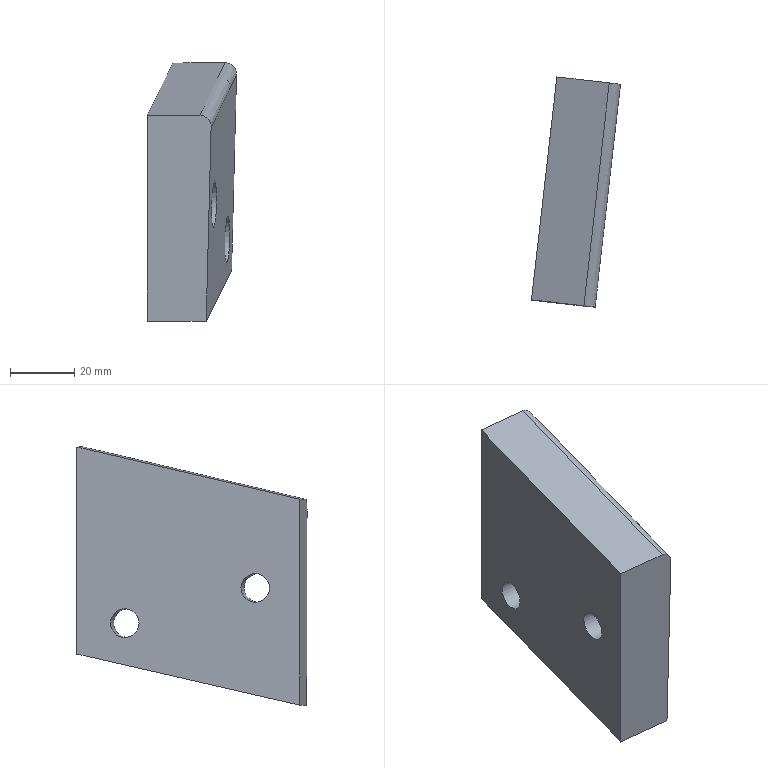Part | NX | features 23 2 | 1 solid | 13 faces | box 27.795 x 71.813 x 80.626 mm | volume 82272 mm3 | plane 7 | cylinder 4 | spline 2 | commonest cylinder face diameters 9 x2 14.5 x2
STEP:
#1=CARTESIAN_POINT('',(2638.723,-314.145,-117.631));
#2=VERTEX_POINT('',#1);
#3=CARTESIAN_POINT('',(2646.647,-244.595,-101.684));
#4=VERTEX_POINT('',#3);
#5=CARTESIAN_POINT('',(2657.951,-145.383,-78.935));
#6=DIRECTION('',(0.1104,0.9687,0.2221));
#7=VECTOR('',#6,1000.);
#8=LINE('',#5,#7);
#9=EDGE_CURVE('',#2,#4,#8,.T.);
#10=ORIENTED_EDGE('',*,*,#9,.T.);
#11=CARTESIAN_POINT('',(2648.194,-244.771,-40.694));
#12=VERTEX_POINT('',#11);
#13=CARTESIAN_POINT('',(2646.722,-244.604,-98.712));
#14=DIRECTION('',(0.02536,-0.002889,0.9997));
#15=VECTOR('',#14,1000.);
#16=LINE('',#13,#15);
#17=EDGE_CURVE('',#4,#12,#16,.T.);
#18=ORIENTED_EDGE('',*,*,#17,.T.);
#19=CARTESIAN_POINT('',(2640.259,-314.32,-57.071));
#20=VERTEX_POINT('',#19);
#21=CARTESIAN_POINT('',(2648.194,-244.771,-40.694));
#22=CARTESIAN_POINT('',(2648.121,-245.409,-40.844));
#23=CARTESIAN_POINT('',(2647.971,-246.727,-41.154));
#24=CARTESIAN_POINT('',(2647.771,-248.484,-41.566));
#25=CARTESIAN_POINT('',(2647.603,-249.954,-41.911));
#26=CARTESIAN_POINT('',(2647.473,-251.092,-42.178));
#27=CARTESIAN_POINT('',(2647.363,-252.06,-42.405));
#28=CARTESIAN_POINT('',(2647.282,-252.767,-42.571));
#29=CARTESIAN_POINT('',(2647.238,-253.152,-42.661));
#30=CARTESIAN_POINT('',(2647.197,-253.509,-42.744));
#31=CARTESIAN_POINT('',(2647.186,-253.611,-42.768));
#32=CARTESIAN_POINT('',(2647.159,-253.849,-42.824));
#33=CARTESIAN_POINT('',(2647.113,-254.247,-42.917));
#34=CARTESIAN_POINT('',(2647.037,-254.913,-43.073));
#35=CARTESIAN_POINT('',(2646.934,-255.821,-43.285));
#36=CARTESIAN_POINT('',(2646.778,-257.19,-43.605));
#37=CARTESIAN_POINT('',(2646.593,-258.809,-43.984));
#38=CARTESIAN_POINT('',(2646.386,-260.625,-44.409));
#39=CARTESIAN_POINT('',(2646.205,-262.211,-44.779));
#40=CARTESIAN_POINT('',(2646.057,-263.51,-45.083));
#41=CARTESIAN_POINT('',(2645.862,-265.219,-45.483));
#42=CARTESIAN_POINT('',(2645.642,-267.144,-45.933));
#43=CARTESIAN_POINT('',(2645.448,-268.843,-46.331));
#44=CARTESIAN_POINT('',(2645.33,-269.883,-46.574));
#45=CARTESIAN_POINT('',(2645.263,-270.472,-46.712));
#46=CARTESIAN_POINT('',(2645.224,-270.807,-46.791));
#47=CARTESIAN_POINT('',(2645.15,-271.46,-46.944));
#48=CARTESIAN_POINT('',(2645.064,-272.21,-47.119));
#49=CARTESIAN_POINT('',(2644.911,-273.556,-47.435));
#50=CARTESIAN_POINT('',(2644.701,-275.393,-47.867));
#51=CARTESIAN_POINT('',(2644.497,-277.181,-48.287));
#52=CARTESIAN_POINT('',(2644.343,-278.535,-48.606));
#53=CARTESIAN_POINT('',(2644.22,-279.609,-48.859));
#54=CARTESIAN_POINT('',(2644.135,-280.355,-49.034));
#55=CARTESIAN_POINT('',(2644.002,-281.523,-49.31));
#56=CARTESIAN_POINT('',(2643.761,-283.631,-49.808));
#57=CARTESIAN_POINT('',(2643.374,-287.024,-50.609));
#58=CARTESIAN_POINT('',(2642.933,-290.886,-51.523));
#59=CARTESIAN_POINT('',(2642.599,-293.818,-52.217));
#60=CARTESIAN_POINT('',(2642.396,-295.596,-52.638));
#61=CARTESIAN_POINT('',(2642.25,-296.876,-52.941));
#62=CARTESIAN_POINT('',(2642.061,-298.527,-53.333));
#63=CARTESIAN_POINT('',(2641.837,-300.493,-53.798));
#64=CARTESIAN_POINT('',(2641.569,-302.845,-54.355));
#65=CARTESIAN_POINT('',(2641.278,-305.392,-54.958));
#66=CARTESIAN_POINT('',(2640.928,-308.459,-55.684));
#67=CARTESIAN_POINT('',(2640.563,-311.658,-56.442));
#68=CARTESIAN_POINT('',(2640.347,-313.545,-56.888));
#69=CARTESIAN_POINT('',(2640.259,-314.32,-57.071));
#70=B_SPLINE_CURVE_WITH_KNOTS('',3,(#21,#22,#23,#24,#25,#26,#27,#28,#29,#30,#31,#32,#33,#34,#35,#36,#37,#38,#39,#40,#41,#42,#43,#44,#45,#46,#47,#48,#49,#50,#51,#52,#53,#54,#55,#56,#57,#58,#59,#60,#61,#62,#63,#64,#65,#66,#67,#68,#69),.UNSPECIFIED.,.F.,.F.,(4,1,1,1,1,1,1,1,1,1,1,1,1,1,1,1,1,1,1,1,1,1,1,1,1,1,1,1,1,1,1,1,1,1,1,1,1,1,1,1,1,1,1,1,1,1,4),(0.,0.03125,0.0625,0.07812,0.09375,0.1094,0.1172,0.1211,0.125,0.1289,0.1328,0.1406,0.1562,0.1719,0.1875,0.2188,0.2344,0.25,0.2656,0.2812,0.3125,0.3438,0.3594,0.3672,0.375,0.3828,0.3906,0.4062,0.4375,0.4688,0.4844,0.5,0.5156,0.5312,0.5625,0.625,0.6875,0.7188,0.7344,0.75,0.7656,0.7812,0.8125,0.8438,0.875,0.9375,1.),.UNSPECIFIED.);
#71=EDGE_CURVE('',#20,#12,#70,.F.);
#72=ORIENTED_EDGE('',*,*,#71,.F.);
#73=CARTESIAN_POINT('',(2639.202,-314.2,-98.722));
#74=DIRECTION('',(0.02536,-0.002889,0.9997));
#75=VECTOR('',#74,1000.);
#76=LINE('',#73,#75);
#77=EDGE_CURVE('',#2,#20,#76,.T.);
#78=ORIENTED_EDGE('',*,*,#77,.F.);
#79=EDGE_LOOP('',(#10,#18,#72,#78));
#80=FACE_BOUND('',#79,.T.);
#81=CARTESIAN_POINT('',(2641.148,-298.71,-88.121));
#82=VERTEX_POINT('',#81);
#83=CARTESIAN_POINT('',(2641.155,-300.332,-81.052));
#84=DIRECTION('',(0.9939,-0.1074,-0.02552));
#85=DIRECTION('',(-0.0008715,0.2236,-0.9747));
#86=AXIS2_PLACEMENT_3D('',#83,#84,#85);
#87=ELLIPSE('',#86,7.252,7.25);
#88=EDGE_CURVE('',#82,#82,#87,.T.);
#89=ORIENTED_EDGE('',*,*,#88,.F.);
#90=EDGE_LOOP('',(#89));
#91=FACE_BOUND('',#90,.T.);
#92=CARTESIAN_POINT('',(2645.274,-257.915,-99.121));
#93=VERTEX_POINT('',#92);
#94=CARTESIAN_POINT('',(2645.28,-259.536,-92.052));
#95=DIRECTION('',(-0.9939,0.1074,0.02552));
#96=DIRECTION('',(-0.0008715,0.2236,-0.9747));
#97=AXIS2_PLACEMENT_3D('',#94,#95,#96);
#98=ELLIPSE('',#97,7.252,7.25);
#99=EDGE_CURVE('',#93,#93,#98,.T.);
#100=ORIENTED_EDGE('',*,*,#99,.T.);
#101=EDGE_LOOP('',(#100));
#102=FACE_BOUND('',#101,.T.);
#103=CARTESIAN_POINT('',(2489.055,-1559.415,-706.392));
#104=DIRECTION('',(0.9939,-0.1074,-0.02552));
#105=DIRECTION('',(-0.02537,0.002816,-0.9997));
#106=AXIS2_PLACEMENT_3D('',#103,#104,#105);
#107=PLANE('',#106);
#108=ADVANCED_FACE('',(#80,#91,#102),#107,.T.);
#109=CARTESIAN_POINT('',(2620.4,-312.058,-117.631));
#110=VERTEX_POINT('',#109);
#111=CARTESIAN_POINT('',(2630.336,-313.19,-117.631));
#112=DIRECTION('',(-0.9936,0.1132,-0.000000001));
#113=VECTOR('',#112,1000.);
#114=LINE('',#111,#113);
#115=EDGE_CURVE('',#2,#110,#114,.T.);
#116=ORIENTED_EDGE('',*,*,#115,.F.);
#117=ORIENTED_EDGE('',*,*,#77,.T.);
#118=CARTESIAN_POINT('',(2636.764,-313.922,-53.382));
#119=VERTEX_POINT('',#118);
#120=CARTESIAN_POINT('',(2636.764,-313.922,-53.382));
#121=CARTESIAN_POINT('',(2637.715,-314.03,-53.377));
#122=CARTESIAN_POINT('',(2639.568,-314.242,-54.211));
#123=CARTESIAN_POINT('',(2640.283,-314.323,-56.116));
#124=CARTESIAN_POINT('',(2640.259,-314.32,-57.071));
#125=B_SPLINE_CURVE_WITH_KNOTS('',3,(#120,#121,#122,#123,#124),.UNSPECIFIED.,.F.,.F.,(4,1,4),(0.,0.002827,0.005655),.UNSPECIFIED.);
#126=EDGE_CURVE('',#119,#20,#125,.T.);
#127=ORIENTED_EDGE('',*,*,#126,.F.);
#128=CARTESIAN_POINT('',(2620.4,-312.058,-53.345));
#129=VERTEX_POINT('',#128);
#130=CARTESIAN_POINT('',(2636.764,-313.922,-53.382));
#131=CARTESIAN_POINT('',(2631.31,-313.301,-53.411));
#132=CARTESIAN_POINT('',(2625.855,-312.679,-53.392));
#133=CARTESIAN_POINT('',(2620.4,-312.058,-53.345));
#134=B_SPLINE_CURVE_WITH_KNOTS('',3,(#130,#131,#132,#133),.UNSPECIFIED.,.F.,.F.,(4,4),(0.,0.01647),.UNSPECIFIED.);
#135=EDGE_CURVE('',#119,#129,#134,.T.);
#136=ORIENTED_EDGE('',*,*,#135,.T.);
#137=CARTESIAN_POINT('',(2620.4,-312.058,-77.534));
#138=DIRECTION('',(-0.000000001,0.,1.));
#139=VECTOR('',#138,1000.);
#140=LINE('',#137,#139);
#141=EDGE_CURVE('',#110,#129,#140,.T.);
#142=ORIENTED_EDGE('',*,*,#141,.F.);
#143=EDGE_LOOP('',(#116,#117,#127,#136,#142));
#144=FACE_BOUND('',#143,.T.);
#145=CARTESIAN_POINT('',(2630.336,-313.19,-98.495));
#146=DIRECTION('',(-0.1132,-0.9936,0.));
#147=DIRECTION('',(-0.9936,0.1132,0.));
#148=AXIS2_PLACEMENT_3D('',#145,#146,#147);
#149=PLANE('',#148);
#150=ADVANCED_FACE('',(#144),#149,.T.);
#151=CARTESIAN_POINT('',(2627.135,-252.94,-92.052));
#152=VERTEX_POINT('',#151);
#153=CARTESIAN_POINT('',(2626.626,-257.411,-92.052));
#154=DIRECTION('',(0.9936,-0.1132,0.000000001));
#155=DIRECTION('',(0.1132,0.9936,0.));
#156=AXIS2_PLACEMENT_3D('',#153,#154,#155);
#157=CIRCLE('',#156,4.5);
#158=EDGE_CURVE('',#152,#152,#157,.T.);
#159=ORIENTED_EDGE('',*,*,#158,.T.);
#160=EDGE_LOOP('',(#159));
#161=FACE_BOUND('',#160,.T.);
#162=CARTESIAN_POINT('',(2622.494,-293.677,-81.052));
#163=VERTEX_POINT('',#162);
#164=CARTESIAN_POINT('',(2621.985,-298.148,-81.052));
#165=DIRECTION('',(0.9936,-0.1132,0.000000001));
#166=DIRECTION('',(0.1132,0.9936,0.));
#167=AXIS2_PLACEMENT_3D('',#164,#165,#166);
#168=CIRCLE('',#167,4.5);
#169=EDGE_CURVE('',#163,#163,#168,.T.);
#170=ORIENTED_EDGE('',*,*,#169,.T.);
#171=EDGE_LOOP('',(#170));
#172=FACE_BOUND('',#171,.T.);
#173=CARTESIAN_POINT('',(2628.324,-242.508,-101.684));
#174=VERTEX_POINT('',#173);
#175=CARTESIAN_POINT('',(2628.324,-242.508,-37.059));
#176=VERTEX_POINT('',#175);
#177=CARTESIAN_POINT('',(2628.324,-242.508,-77.534));
#178=DIRECTION('',(-0.000000001,0.,1.));
#179=VECTOR('',#178,1000.);
#180=LINE('',#177,#179);
#181=EDGE_CURVE('',#174,#176,#180,.T.);
#182=ORIENTED_EDGE('',*,*,#181,.F.);
#183=CARTESIAN_POINT('',(2624.635,-274.889,-109.109));
#184=DIRECTION('',(0.1104,0.9687,0.2221));
#185=VECTOR('',#184,1000.);
#186=LINE('',#183,#185);
#187=EDGE_CURVE('',#110,#174,#186,.T.);
#188=ORIENTED_EDGE('',*,*,#187,.F.);
#189=ORIENTED_EDGE('',*,*,#141,.T.);
#190=CARTESIAN_POINT('',(2628.324,-242.508,-37.059));
#191=CARTESIAN_POINT('',(2627.663,-248.306,-38.406));
#192=CARTESIAN_POINT('',(2626.341,-259.917,-41.034));
#193=CARTESIAN_POINT('',(2623.701,-283.087,-46.522));
#194=CARTESIAN_POINT('',(2621.72,-300.469,-50.618));
#195=CARTESIAN_POINT('',(2620.4,-312.058,-53.345));
#196=B_SPLINE_CURVE_WITH_KNOTS('',3,(#190,#191,#192,#193,#194,#195),.UNSPECIFIED.,.F.,.F.,(4,1,1,4),(0.000000002,0.01797,0.03593,0.07187),.UNSPECIFIED.);
#197=EDGE_CURVE('',#176,#129,#196,.T.);
#198=ORIENTED_EDGE('',*,*,#197,.F.);
#199=EDGE_LOOP('',(#182,#188,#189,#198));
#200=FACE_BOUND('',#199,.T.);
#201=CARTESIAN_POINT('',(2623.82,-282.036,-77.534));
#202=DIRECTION('',(0.9936,-0.1132,0.000000001));
#203=DIRECTION('',(-0.1132,-0.9936,0.));
#204=AXIS2_PLACEMENT_3D('',#201,#202,#203);
#205=PLANE('',#204);
#206=ADVANCED_FACE('',(#161,#172,#200),#205,.F.);
#207=CARTESIAN_POINT('',(2644.678,-244.371,-37.006));
#208=VERTEX_POINT('',#207);
#209=CARTESIAN_POINT('',(2636.764,-313.922,-53.382));
#210=CARTESIAN_POINT('',(2638.082,-302.336,-50.646));
#211=CARTESIAN_POINT('',(2640.727,-279.163,-45.124));
#212=CARTESIAN_POINT('',(2643.34,-255.967,-39.737));
#213=CARTESIAN_POINT('',(2644.678,-244.371,-37.006));
#214=B_SPLINE_CURVE_WITH_KNOTS('',3,(#209,#210,#211,#212,#213),.UNSPECIFIED.,.F.,.F.,(4,1,4),(0.,0.5,1.),.UNSPECIFIED.);
#215=EDGE_CURVE('',#208,#119,#214,.F.);
#216=ORIENTED_EDGE('',*,*,#215,.F.);
#217=CARTESIAN_POINT('',(2628.324,-242.508,-37.059));
#218=CARTESIAN_POINT('',(2633.775,-243.129,-37.117));
#219=CARTESIAN_POINT('',(2639.227,-243.75,-37.071));
#220=CARTESIAN_POINT('',(2644.678,-244.371,-37.006));
#221=B_SPLINE_CURVE_WITH_KNOTS('',3,(#217,#218,#219,#220),.UNSPECIFIED.,.F.,.F.,(4,4),(0.,0.01646),.UNSPECIFIED.);
#222=EDGE_CURVE('',#176,#208,#221,.T.);
#223=ORIENTED_EDGE('',*,*,#222,.F.);
#224=ORIENTED_EDGE('',*,*,#197,.T.);
#225=ORIENTED_EDGE('',*,*,#135,.F.);
#226=EDGE_LOOP('',(#216,#223,#224,#225));
#227=FACE_BOUND('',#226,.T.);
#228=CARTESIAN_POINT('',(2644.824,-243.965,-36.906));
#229=CARTESIAN_POINT('',(2644.153,-249.833,-38.289));
#230=CARTESIAN_POINT('',(2643.486,-255.702,-39.662));
#231=CARTESIAN_POINT('',(2642.16,-267.439,-42.407));
#232=CARTESIAN_POINT('',(2641.507,-273.309,-43.776));
#233=CARTESIAN_POINT('',(2640.197,-285.036,-46.537));
#234=CARTESIAN_POINT('',(2639.534,-290.893,-47.936));
#235=CARTESIAN_POINT('',(2638.207,-302.63,-50.718));
#236=CARTESIAN_POINT('',(2637.547,-308.495,-52.095));
#237=CARTESIAN_POINT('',(2636.886,-314.358,-53.479));
#238=CARTESIAN_POINT('',(2642.06,-243.64,-36.937));
#239=CARTESIAN_POINT('',(2641.388,-249.513,-38.32));
#240=CARTESIAN_POINT('',(2640.719,-255.386,-39.686));
#241=CARTESIAN_POINT('',(2639.393,-267.125,-42.423));
#242=CARTESIAN_POINT('',(2638.747,-272.992,-43.795));
#243=CARTESIAN_POINT('',(2637.441,-284.719,-46.561));
#244=CARTESIAN_POINT('',(2636.768,-290.578,-47.959));
#245=CARTESIAN_POINT('',(2635.44,-302.314,-50.736));
#246=CARTESIAN_POINT('',(2634.787,-308.182,-52.111));
#247=CARTESIAN_POINT('',(2634.124,-314.045,-53.494));
#248=CARTESIAN_POINT('',(2639.303,-243.311,-36.973));
#249=CARTESIAN_POINT('',(2638.631,-249.192,-38.36));
#250=CARTESIAN_POINT('',(2637.957,-255.074,-39.718));
#251=CARTESIAN_POINT('',(2636.624,-266.814,-42.437));
#252=CARTESIAN_POINT('',(2635.971,-272.67,-43.814));
#253=CARTESIAN_POINT('',(2634.658,-284.398,-46.591));
#254=CARTESIAN_POINT('',(2633.99,-290.265,-47.98));
#255=CARTESIAN_POINT('',(2632.667,-301.996,-50.751));
#256=CARTESIAN_POINT('',(2632.013,-307.864,-52.135));
#257=CARTESIAN_POINT('',(2631.351,-313.73,-53.515));
#258=CARTESIAN_POINT('',(2633.743,-242.67,-36.996));
#259=CARTESIAN_POINT('',(2633.063,-248.562,-38.386));
#260=CARTESIAN_POINT('',(2632.386,-254.454,-39.727));
#261=CARTESIAN_POINT('',(2631.065,-266.197,-42.423));
#262=CARTESIAN_POINT('',(2630.408,-272.043,-43.802));
#263=CARTESIAN_POINT('',(2629.085,-283.771,-46.587));
#264=CARTESIAN_POINT('',(2628.422,-289.645,-47.969));
#265=CARTESIAN_POINT('',(2627.101,-301.374,-50.733));
#266=CARTESIAN_POINT('',(2626.442,-307.24,-52.12));
#267=CARTESIAN_POINT('',(2625.784,-313.109,-53.499));
#268=CARTESIAN_POINT('',(2630.954,-242.362,-36.984));
#269=CARTESIAN_POINT('',(2630.266,-248.263,-38.365));
#270=CARTESIAN_POINT('',(2629.593,-254.148,-39.695));
#271=CARTESIAN_POINT('',(2628.293,-265.886,-42.401));
#272=CARTESIAN_POINT('',(2627.64,-271.737,-43.783));
#273=CARTESIAN_POINT('',(2626.315,-283.468,-46.562));
#274=CARTESIAN_POINT('',(2625.652,-289.342,-47.94));
#275=CARTESIAN_POINT('',(2624.332,-301.068,-50.702));
#276=CARTESIAN_POINT('',(2623.674,-306.934,-52.092));
#277=CARTESIAN_POINT('',(2623.015,-312.803,-53.472));
#278=CARTESIAN_POINT('',(2628.172,-242.061,-36.958));
#279=CARTESIAN_POINT('',(2627.49,-247.964,-38.331));
#280=CARTESIAN_POINT('',(2626.826,-253.843,-39.659));
#281=CARTESIAN_POINT('',(2625.527,-265.576,-42.379));
#282=CARTESIAN_POINT('',(2624.872,-271.431,-43.763));
#283=CARTESIAN_POINT('',(2623.55,-283.164,-46.539));
#284=CARTESIAN_POINT('',(2622.891,-289.035,-47.917));
#285=CARTESIAN_POINT('',(2621.572,-300.763,-50.681));
#286=CARTESIAN_POINT('',(2620.91,-306.628,-52.07));
#287=CARTESIAN_POINT('',(2620.251,-312.497,-53.451));
#288=B_SPLINE_SURFACE_WITH_KNOTS('',3,3,((#228,#229,#230,#231,#232,#233,#234,#235,#236,#237),(#238,#239,#240,#241,#242,#243,#244,#245,#246,#247),(#248,#249,#250,#251,#252,#253,#254,#255,#256,#257),(#258,#259,#260,#261,#262,#263,#264,#265,#266,#267),(#268,#269,#270,#271,#272,#273,#274,#275,#276,#277),(#278,#279,#280,#281,#282,#283,#284,#285,#286,#287)),.UNSPECIFIED.,.F.,.F.,.F.,(4,2,4),(4,2,2,2,4),(0.0002852,0.5,1.),(0.00000002,0.25,0.5,0.75,1.),.UNSPECIFIED.);
#289=ADVANCED_FACE('',(#227),#288,.T.);
#290=CARTESIAN_POINT('',(2644.678,-244.371,-37.006));
#291=CARTESIAN_POINT('',(2645.631,-244.479,-36.994));
#292=CARTESIAN_POINT('',(2647.497,-244.692,-37.823));
#293=CARTESIAN_POINT('',(2648.218,-244.774,-39.735));
#294=CARTESIAN_POINT('',(2648.194,-244.771,-40.694));
#295=B_SPLINE_CURVE_WITH_KNOTS('',3,(#290,#291,#292,#293,#294),.UNSPECIFIED.,.F.,.F.,(4,1,4),(0.,0.002838,0.005676),.UNSPECIFIED.);
#296=EDGE_CURVE('',#208,#12,#295,.T.);
#297=ORIENTED_EDGE('',*,*,#296,.F.);
#298=ORIENTED_EDGE('',*,*,#215,.T.);
#299=ORIENTED_EDGE('',*,*,#126,.T.);
#300=ORIENTED_EDGE('',*,*,#71,.T.);
#301=EDGE_LOOP('',(#297,#298,#299,#300));
#302=FACE_BOUND('',#301,.T.);
#303=CARTESIAN_POINT('',(2644.696,-243.944,-36.906));
#304=CARTESIAN_POINT('',(2645.118,-243.994,-36.902));
#305=CARTESIAN_POINT('',(2645.577,-244.031,-36.967));
#306=CARTESIAN_POINT('',(2646.475,-244.054,-37.304));
#307=CARTESIAN_POINT('',(2646.911,-244.04,-37.574));
#308=CARTESIAN_POINT('',(2647.629,-243.958,-38.27));
#309=CARTESIAN_POINT('',(2647.91,-243.89,-38.694));
#310=CARTESIAN_POINT('',(2648.264,-243.724,-39.57));
#311=CARTESIAN_POINT('',(2648.335,-243.626,-40.019));
#312=CARTESIAN_POINT('',(2648.335,-243.529,-40.433));
#313=CARTESIAN_POINT('',(2643.344,-255.807,-39.701));
#314=CARTESIAN_POINT('',(2643.767,-255.856,-39.696));
#315=CARTESIAN_POINT('',(2644.225,-255.893,-39.761));
#316=CARTESIAN_POINT('',(2645.123,-255.917,-40.098));
#317=CARTESIAN_POINT('',(2645.558,-255.903,-40.368));
#318=CARTESIAN_POINT('',(2646.276,-255.822,-41.064));
#319=CARTESIAN_POINT('',(2646.556,-255.755,-41.488));
#320=CARTESIAN_POINT('',(2646.91,-255.59,-42.365));
#321=CARTESIAN_POINT('',(2646.981,-255.494,-42.813));
#322=CARTESIAN_POINT('',(2646.981,-255.397,-43.228));
#323=CARTESIAN_POINT('',(2642.009,-267.682,-42.454));
#324=CARTESIAN_POINT('',(2642.43,-267.73,-42.452));
#325=CARTESIAN_POINT('',(2642.887,-267.767,-42.519));
#326=CARTESIAN_POINT('',(2643.78,-267.79,-42.859));
#327=CARTESIAN_POINT('',(2644.213,-267.776,-43.13));
#328=CARTESIAN_POINT('',(2644.927,-267.695,-43.826));
#329=CARTESIAN_POINT('',(2645.205,-267.629,-44.249));
#330=CARTESIAN_POINT('',(2645.556,-267.466,-45.123));
#331=CARTESIAN_POINT('',(2645.627,-267.37,-45.57));
#332=CARTESIAN_POINT('',(2645.627,-267.274,-45.983));
#333=CARTESIAN_POINT('',(2639.966,-285.496,-46.653));
#334=CARTESIAN_POINT('',(2640.388,-285.545,-46.649));
#335=CARTESIAN_POINT('',(2640.845,-285.582,-46.715));
#336=CARTESIAN_POINT('',(2641.741,-285.604,-47.053));
#337=CARTESIAN_POINT('',(2642.176,-285.59,-47.323));
#338=CARTESIAN_POINT('',(2642.892,-285.506,-48.019));
#339=CARTESIAN_POINT('',(2643.172,-285.438,-48.442));
#340=CARTESIAN_POINT('',(2643.525,-285.271,-49.317));
#341=CARTESIAN_POINT('',(2643.596,-285.173,-49.764));
#342=CARTESIAN_POINT('',(2643.596,-285.075,-50.178));
#343=CARTESIAN_POINT('',(2639.292,-291.43,-48.071));
#344=CARTESIAN_POINT('',(2639.714,-291.479,-48.068));
#345=CARTESIAN_POINT('',(2640.171,-291.515,-48.134));
#346=CARTESIAN_POINT('',(2641.066,-291.536,-48.473));
#347=CARTESIAN_POINT('',(2641.5,-291.522,-48.743));
#348=CARTESIAN_POINT('',(2642.216,-291.437,-49.438));
#349=CARTESIAN_POINT('',(2642.495,-291.369,-49.861));
#350=CARTESIAN_POINT('',(2642.848,-291.2,-50.735));
#351=CARTESIAN_POINT('',(2642.919,-291.102,-51.182));
#352=CARTESIAN_POINT('',(2642.919,-291.004,-51.595));
#353=CARTESIAN_POINT('',(2637.945,-303.285,-50.878));
#354=CARTESIAN_POINT('',(2638.366,-303.333,-50.876));
#355=CARTESIAN_POINT('',(2638.822,-303.37,-50.943));
#356=CARTESIAN_POINT('',(2639.717,-303.392,-51.282));
#357=CARTESIAN_POINT('',(2640.149,-303.378,-51.553));
#358=CARTESIAN_POINT('',(2640.864,-303.295,-52.249));
#359=CARTESIAN_POINT('',(2641.142,-303.228,-52.671));
#360=CARTESIAN_POINT('',(2641.494,-303.062,-53.545));
#361=CARTESIAN_POINT('',(2641.565,-302.965,-53.992));
#362=CARTESIAN_POINT('',(2641.565,-302.868,-54.405));
#363=CARTESIAN_POINT('',(2637.269,-309.22,-52.272));
#364=CARTESIAN_POINT('',(2637.69,-309.268,-52.269));
#365=CARTESIAN_POINT('',(2638.147,-309.305,-52.336));
#366=CARTESIAN_POINT('',(2639.04,-309.327,-52.676));
#367=CARTESIAN_POINT('',(2639.473,-309.312,-52.947));
#368=CARTESIAN_POINT('',(2640.187,-309.23,-53.642));
#369=CARTESIAN_POINT('',(2640.465,-309.162,-54.065));
#370=CARTESIAN_POINT('',(2640.817,-308.997,-54.939));
#371=CARTESIAN_POINT('',(2640.888,-308.9,-55.385));
#372=CARTESIAN_POINT('',(2640.888,-308.803,-55.798));
#373=CARTESIAN_POINT('',(2636.594,-315.156,-53.674));
#374=CARTESIAN_POINT('',(2637.015,-315.204,-53.672));
#375=CARTESIAN_POINT('',(2637.471,-315.24,-53.739));
#376=CARTESIAN_POINT('',(2638.364,-315.262,-54.079));
#377=CARTESIAN_POINT('',(2638.797,-315.247,-54.35));
#378=CARTESIAN_POINT('',(2639.51,-315.165,-55.045));
#379=CARTESIAN_POINT('',(2639.789,-315.097,-55.467));
#380=CARTESIAN_POINT('',(2640.14,-314.93,-56.341));
#381=CARTESIAN_POINT('',(2640.211,-314.833,-56.787));
#382=CARTESIAN_POINT('',(2640.211,-314.735,-57.2));
#383=B_SPLINE_SURFACE_WITH_KNOTS('',3,3,((#303,#304,#305,#306,#307,#308,#309,#310,#311,#312),(#313,#314,#315,#316,#317,#318,#319,#320,#321,#322),(#323,#324,#325,#326,#327,#328,#329,#330,#331,#332),(#333,#334,#335,#336,#337,#338,#339,#340,#341,#342),(#343,#344,#345,#346,#347,#348,#349,#350,#351,#352),(#353,#354,#355,#356,#357,#358,#359,#360,#361,#362),(#363,#364,#365,#366,#367,#368,#369,#370,#371,#372),(#373,#374,#375,#376,#377,#378,#379,#380,#381,#382)),.UNSPECIFIED.,.F.,.F.,.F.,(4,2,2,4),(4,2,2,2,4),(0.,0.5,0.75,1.),(-0.006002,0.247,0.5,0.753,1.006),.UNSPECIFIED.);
#384=ADVANCED_FACE('',(#302),#383,.T.);
#385=ORIENTED_EDGE('',*,*,#17,.F.);
#386=CARTESIAN_POINT('',(2638.26,-243.64,-101.684));
#387=DIRECTION('',(0.9936,-0.1132,0.000000001));
#388=VECTOR('',#387,1000.);
#389=LINE('',#386,#388);
#390=EDGE_CURVE('',#174,#4,#389,.T.);
#391=ORIENTED_EDGE('',*,*,#390,.F.);
#392=ORIENTED_EDGE('',*,*,#181,.T.);
#393=ORIENTED_EDGE('',*,*,#222,.T.);
#394=ORIENTED_EDGE('',*,*,#296,.T.);
#395=EDGE_LOOP('',(#385,#391,#392,#393,#394));
#396=FACE_BOUND('',#395,.T.);
#397=CARTESIAN_POINT('',(2638.26,-243.64,-98.495));
#398=DIRECTION('',(-0.1132,-0.9936,0.));
#399=DIRECTION('',(-0.9936,0.1132,0.));
#400=AXIS2_PLACEMENT_3D('',#397,#398,#399);
#401=PLANE('',#400);
#402=ADVANCED_FACE('',(#396),#401,.F.);
#403=CARTESIAN_POINT('',(2630.417,-303.638,-81.052));
#404=VERTEX_POINT('',#403);
#405=CARTESIAN_POINT('',(2630.927,-299.166,-81.052));
#406=DIRECTION('',(0.9936,-0.1132,0.000000001));
#407=DIRECTION('',(-0.1132,-0.9936,0.));
#408=AXIS2_PLACEMENT_3D('',#405,#406,#407);
#409=CIRCLE('',#408,4.5);
#410=EDGE_CURVE('',#404,#404,#409,.T.);
#411=ORIENTED_EDGE('',*,*,#410,.T.);
#412=EDGE_LOOP('',(#411));
#413=FACE_BOUND('',#412,.T.);
#414=ORIENTED_EDGE('',*,*,#169,.F.);
#415=EDGE_LOOP('',(#414));
#416=FACE_BOUND('',#415,.T.);
#417=CARTESIAN_POINT('',(2641.856,-300.412,-81.052));
#418=DIRECTION('',(-0.9936,0.1132,-0.000000001));
#419=DIRECTION('',(-0.01281,-0.1125,-0.9936));
#420=AXIS2_PLACEMENT_3D('',#417,#418,#419);
#421=CYLINDRICAL_SURFACE('',#420,4.5);
#422=ADVANCED_FACE('',(#413,#416),#421,.F.);
#423=ORIENTED_EDGE('',*,*,#410,.F.);
#424=EDGE_LOOP('',(#423));
#425=FACE_BOUND('',#424,.T.);
#426=CARTESIAN_POINT('',(2631.02,-298.351,-73.849));
#427=VERTEX_POINT('',#426);
#428=CARTESIAN_POINT('',(2630.927,-299.166,-81.052));
#429=DIRECTION('',(0.9936,-0.1132,0.000000001));
#430=DIRECTION('',(0.01281,0.1125,0.9936));
#431=AXIS2_PLACEMENT_3D('',#428,#429,#430);
#432=CIRCLE('',#431,7.25);
#433=EDGE_CURVE('',#427,#427,#432,.T.);
#434=ORIENTED_EDGE('',*,*,#433,.T.);
#435=EDGE_LOOP('',(#434));
#436=FACE_BOUND('',#435,.T.);
#437=CARTESIAN_POINT('',(2630.927,-299.166,-81.052));
#438=DIRECTION('',(-0.9936,0.1132,-0.000000001));
#439=DIRECTION('',(0.1132,0.9936,0.));
#440=AXIS2_PLACEMENT_3D('',#437,#438,#439);
#441=PLANE('',#440);
#442=ADVANCED_FACE('',(#425,#436),#441,.F.);
#443=ORIENTED_EDGE('',*,*,#433,.F.);
#444=EDGE_LOOP('',(#443));
#445=FACE_BOUND('',#444,.T.);
#446=ORIENTED_EDGE('',*,*,#88,.T.);
#447=EDGE_LOOP('',(#446));
#448=FACE_BOUND('',#447,.T.);
#449=CARTESIAN_POINT('',(2641.856,-300.412,-81.052));
#450=DIRECTION('',(-0.9936,0.1132,-0.000000001));
#451=DIRECTION('',(-0.01281,-0.1125,-0.9936));
#452=AXIS2_PLACEMENT_3D('',#449,#450,#451);
#453=CYLINDRICAL_SURFACE('',#452,7.25);
#454=ADVANCED_FACE('',(#445,#448),#453,.F.);
#455=CARTESIAN_POINT('',(2636.078,-253.959,-92.052));
#456=VERTEX_POINT('',#455);
#457=CARTESIAN_POINT('',(2635.568,-258.43,-92.052));
#458=DIRECTION('',(-0.9936,0.1132,-0.000000001));
#459=DIRECTION('',(0.1132,0.9936,0.));
#460=AXIS2_PLACEMENT_3D('',#457,#458,#459);
#461=CIRCLE('',#460,4.5);
#462=EDGE_CURVE('',#456,#456,#461,.T.);
#463=ORIENTED_EDGE('',*,*,#462,.F.);
#464=EDGE_LOOP('',(#463));
#465=FACE_BOUND('',#464,.T.);
#466=ORIENTED_EDGE('',*,*,#158,.F.);
#467=EDGE_LOOP('',(#466));
#468=FACE_BOUND('',#467,.T.);
#469=CARTESIAN_POINT('',(2646.497,-259.675,-92.052));
#470=DIRECTION('',(-0.9936,0.1132,-0.000000001));
#471=DIRECTION('',(0.01281,0.1125,-0.9936));
#472=AXIS2_PLACEMENT_3D('',#469,#470,#471);
#473=CYLINDRICAL_SURFACE('',#472,4.5);
#474=ADVANCED_FACE('',(#465,#468),#473,.F.);
#475=ORIENTED_EDGE('',*,*,#462,.T.);
#476=EDGE_LOOP('',(#475));
#477=FACE_BOUND('',#476,.T.);
#478=CARTESIAN_POINT('',(2635.475,-259.245,-84.849));
#479=VERTEX_POINT('',#478);
#480=CARTESIAN_POINT('',(2635.568,-258.43,-92.052));
#481=DIRECTION('',(-0.9936,0.1132,-0.000000001));
#482=DIRECTION('',(-0.01281,-0.1125,0.9936));
#483=AXIS2_PLACEMENT_3D('',#480,#481,#482);
#484=CIRCLE('',#483,7.25);
#485=EDGE_CURVE('',#479,#479,#484,.T.);
#486=ORIENTED_EDGE('',*,*,#485,.F.);
#487=EDGE_LOOP('',(#486));
#488=FACE_BOUND('',#487,.T.);
#489=CARTESIAN_POINT('',(2635.568,-258.43,-92.052));
#490=DIRECTION('',(-0.9936,0.1132,-0.000000001));
#491=DIRECTION('',(-0.1132,-0.9936,0.));
#492=AXIS2_PLACEMENT_3D('',#489,#490,#491);
#493=PLANE('',#492);
#494=ADVANCED_FACE('',(#477,#488),#493,.F.);
#495=ORIENTED_EDGE('',*,*,#485,.T.);
#496=EDGE_LOOP('',(#495));
#497=FACE_BOUND('',#496,.T.);
#498=ORIENTED_EDGE('',*,*,#99,.F.);
#499=EDGE_LOOP('',(#498));
#500=FACE_BOUND('',#499,.T.);
#501=CARTESIAN_POINT('',(2646.497,-259.675,-92.052));
#502=DIRECTION('',(-0.9936,0.1132,-0.000000001));
#503=DIRECTION('',(0.01281,0.1125,-0.9936));
#504=AXIS2_PLACEMENT_3D('',#501,#502,#503);
#505=CYLINDRICAL_SURFACE('',#504,7.25);
#506=ADVANCED_FACE('',(#497,#500),#505,.F.);
#507=ORIENTED_EDGE('',*,*,#9,.F.);
#508=ORIENTED_EDGE('',*,*,#115,.T.);
#509=ORIENTED_EDGE('',*,*,#187,.T.);
#510=ORIENTED_EDGE('',*,*,#390,.T.);
#511=EDGE_LOOP('',(#507,#508,#509,#510));
#512=FACE_BOUND('',#511,.T.);
#513=CARTESIAN_POINT('',(-2624.08,456.429,-78.935));
#514=DIRECTION('',(-0.02515,-0.2207,0.975));
#515=DIRECTION('',(0.,0.9753,0.2208));
#516=AXIS2_PLACEMENT_3D('',#513,#514,#515);
#517=PLANE('',#516);
#518=ADVANCED_FACE('',(#512),#517,.F.);
#519=CLOSED_SHELL('',(#108,#150,#206,#289,#384,#402,#422,#442,#454,#474,#494,#506,#518));
#520=MANIFOLD_SOLID_BREP('',#519);
#521=(LENGTH_UNIT()NAMED_UNIT(*)SI_UNIT(.MILLI.,.METRE.));
#522=UNCERTAINTY_MEASURE_WITH_UNIT(LENGTH_MEASURE(0.08945),#521,'','');
#523=(NAMED_UNIT(*)PLANE_ANGLE_UNIT()SI_UNIT($,.RADIAN.));
#524=(NAMED_UNIT(*)SI_UNIT($,.STERADIAN.)SOLID_ANGLE_UNIT());
#525=(GEOMETRIC_REPRESENTATION_CONTEXT(3)GLOBAL_UNCERTAINTY_ASSIGNED_CONTEXT((#522))GLOBAL_UNIT_ASSIGNED_CONTEXT((#521,#523,#524))REPRESENTATION_CONTEXT('',''));
#526=ADVANCED_BREP_SHAPE_REPRESENTATION('',(#520),#525);